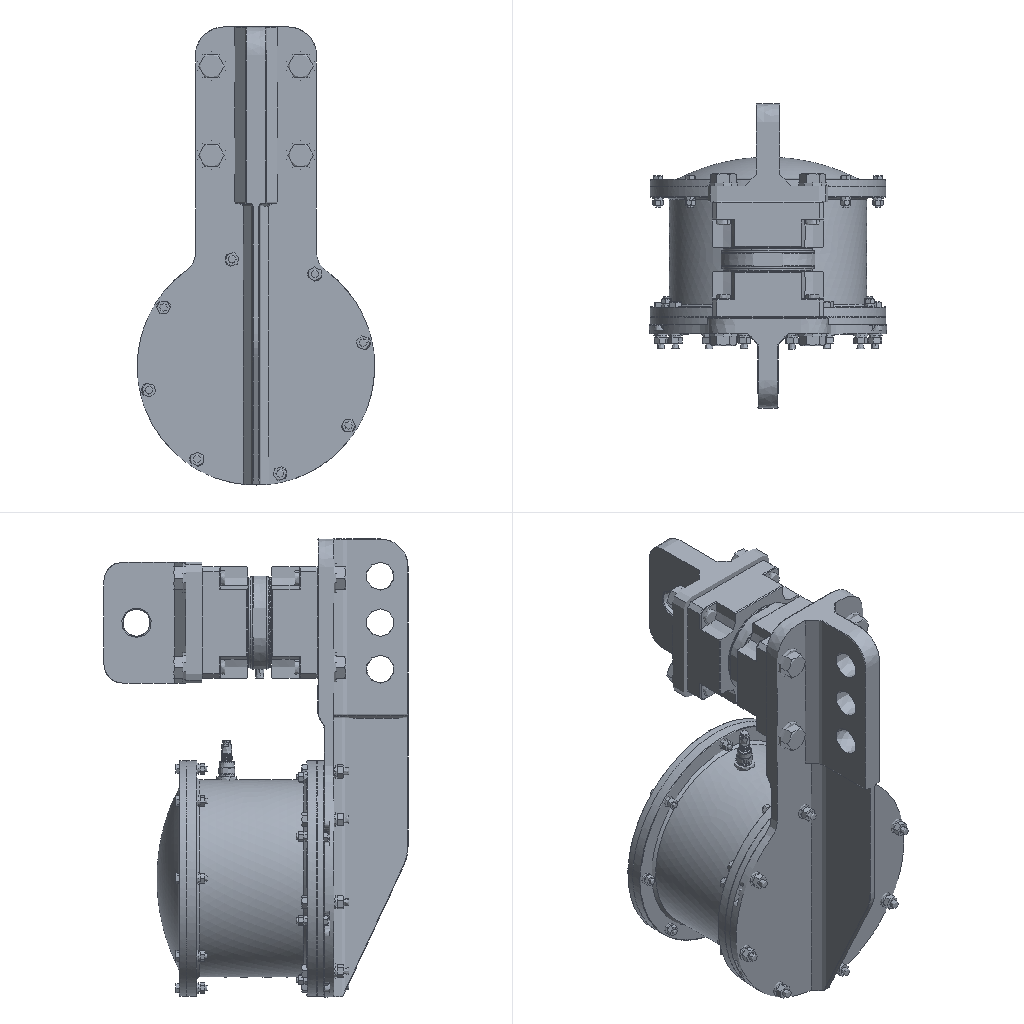Simulation study | ansys workbench
Set-up summary, first 219 of 917 lines:
category,name,step,type,value,unit,region
solver,ansys_mapdl
solver,version,,,22.2
units,MPA,,stated
analysis,deck,,static,static
load_step,requested,,,1
analysis,nlgeom,,,False
mesh,nodes,,,682109
mesh,elements,,,699995
element_type,ANSYS 187 (type 1),,solid,183
element_type,ANSYS 187 (type 2),,solid,17706
element_type,ANSYS 187 (type 3),,solid,59015
element_type,ANSYS 187 (type 4),,solid,6630
element_type,ANSYS 187 (type 5),,solid,23158
element_type,ANSYS 187 (type 6),,solid,2789
element_type,ANSYS 187 (type 7),,solid,7418
element_type,ANSYS 187 (type 8),,solid,4974
element_type,ANSYS 187 (type 9),,solid,5394
element_type,ANSYS 187 (type 10),,solid,2967
element_type,ANSYS 187 (type 11),,solid,1024
element_type,ANSYS 187 (type 12),,solid,918
element_type,ANSYS 187 (type 13),,solid,65195
element_type,ANSYS 187 (type 14),,solid,743
element_type,ANSYS 187 (type 15),,solid,719
element_type,ANSYS 187 (type 16),,solid,743
element_type,ANSYS 187 (type 17),,solid,716
element_type,ANSYS 187 (type 18),,solid,131786
element_type,ANSYS 187 (type 19),,solid,1036
element_type,ANSYS 187 (type 20),,solid,935
element_type,ANSYS 187 (type 21),,solid,48
element_type,ANSYS 187 (type 22),,solid,56
element_type,ANSYS 187 (type 23),,solid,234
element_type,ANSYS 187 (type 24),,solid,596
element_type,ANSYS 187 (type 25),,solid,599
element_type,ANSYS 187 (type 26),,solid,56
element_type,ANSYS 187 (type 27),,solid,48
element_type,ANSYS 187 (type 28),,solid,249
element_type,ANSYS 187 (type 29),,solid,561
element_type,ANSYS 187 (type 30),,solid,56
element_type,ANSYS 187 (type 31),,solid,48
element_type,ANSYS 187 (type 32),,solid,257
element_type,ANSYS 187 (type 33),,solid,588
element_type,ANSYS 187 (type 34),,solid,56
element_type,ANSYS 187 (type 35),,solid,48
element_type,ANSYS 187 (type 36),,solid,260
element_type,ANSYS 187 (type 37),,solid,577
element_type,ANSYS 187 (type 38),,solid,56
element_type,ANSYS 187 (type 39),,solid,48
element_type,ANSYS 187 (type 40),,solid,228
element_type,ANSYS 187 (type 41),,solid,659
element_type,ANSYS 187 (type 42),,solid,56
element_type,ANSYS 187 (type 43),,solid,48
element_type,ANSYS 187 (type 44),,solid,222
element_type,ANSYS 187 (type 45),,solid,586
element_type,ANSYS 187 (type 46),,solid,56
element_type,ANSYS 187 (type 47),,solid,48
element_type,ANSYS 187 (type 48),,solid,258
element_type,ANSYS 187 (type 49),,solid,593
element_type,ANSYS 187 (type 50),,solid,56
element_type,ANSYS 187 (type 51),,solid,48
element_type,ANSYS 187 (type 52),,solid,245
element_type,ANSYS 187 (type 53),,solid,215
element_type,ANSYS 187 (type 54),,solid,586
element_type,ANSYS 187 (type 55),,solid,58
element_type,ANSYS 187 (type 56),,solid,42
element_type,ANSYS 187 (type 57),,solid,47283
element_type,ANSYS 187 (type 58),,solid,647
element_type,ANSYS 187 (type 59),,solid,54
element_type,ANSYS 187 (type 60),,solid,54
element_type,ANSYS 187 (type 61),,solid,660
element_type,ANSYS 187 (type 62),,solid,54
element_type,ANSYS 187 (type 63),,solid,653
element_type,ANSYS 187 (type 64),,solid,54
element_type,ANSYS 187 (type 65),,solid,669
element_type,ANSYS 187 (type 66),,solid,670
element_type,ANSYS 187 (type 67),,solid,690
element_type,ANSYS 187 (type 68),,solid,661
element_type,ANSYS 187 (type 69),,solid,682
element_type,ANSYS 187 (type 70),,solid,48
element_type,ANSYS 187 (type 71),,solid,48
element_type,ANSYS 187 (type 72),,solid,48
element_type,ANSYS 187 (type 73),,solid,48
element_type,ANSYS 187 (type 74),,solid,554
element_type,ANSYS 187 (type 75),,solid,51
element_type,ANSYS 187 (type 76),,solid,48
element_type,ANSYS 187 (type 77),,solid,251
element_type,ANSYS 187 (type 78),,solid,48
element_type,ANSYS 187 (type 79),,solid,227
element_type,ANSYS 187 (type 80),,solid,51
element_type,ANSYS 187 (type 81),,solid,601
element_type,ANSYS 187 (type 82),,solid,48
element_type,ANSYS 187 (type 83),,solid,269
element_type,ANSYS 187 (type 84),,solid,51
element_type,ANSYS 187 (type 85),,solid,602
element_type,ANSYS 187 (type 86),,solid,48
element_type,ANSYS 187 (type 87),,solid,246
element_type,ANSYS 187 (type 88),,solid,51
element_type,ANSYS 187 (type 89),,solid,677
element_type,ANSYS 187 (type 90),,solid,48
element_type,ANSYS 187 (type 91),,solid,236
element_type,ANSYS 187 (type 92),,solid,51
element_type,ANSYS 187 (type 93),,solid,543
element_type,ANSYS 187 (type 94),,solid,48
element_type,ANSYS 187 (type 95),,solid,251
element_type,ANSYS 187 (type 96),,solid,51
element_type,ANSYS 187 (type 97),,solid,632
element_type,ANSYS 187 (type 98),,solid,48
element_type,ANSYS 187 (type 99),,solid,204
element_type,ANSYS 187 (type 100),,solid,51
element_type,ANSYS 187 (type 101),,solid,593
element_type,ANSYS 187 (type 102),,solid,48
element_type,ANSYS 187 (type 103),,solid,250
element_type,ANSYS 187 (type 104),,solid,51
element_type,ANSYS 187 (type 105),,solid,644
element_type,ANSYS 187 (type 106),,solid,233
element_type,ANSYS 187 (type 107),,solid,561
element_type,ANSYS 187 (type 108),,solid,42
element_type,ANSYS 187 (type 109),,solid,56
element_type,ANSYS 187 (type 110),,solid,261
element_type,ANSYS 187 (type 111),,solid,546
element_type,ANSYS 187 (type 112),,solid,42
element_type,ANSYS 187 (type 113),,solid,58
element_type,ANSYS 187 (type 114),,solid,217
element_type,ANSYS 187 (type 115),,solid,595
element_type,ANSYS 187 (type 116),,solid,42
element_type,ANSYS 187 (type 117),,solid,56
element_type,ANSYS 187 (type 118),,solid,218
element_type,ANSYS 187 (type 119),,solid,571
element_type,ANSYS 187 (type 120),,solid,42
element_type,ANSYS 187 (type 121),,solid,63
element_type,ANSYS 187 (type 122),,solid,222
element_type,ANSYS 187 (type 123),,solid,549
element_type,ANSYS 187 (type 124),,solid,42
element_type,ANSYS 187 (type 125),,solid,57
element_type,ANSYS 187 (type 126),,solid,236
element_type,ANSYS 187 (type 127),,solid,580
element_type,ANSYS 187 (type 128),,solid,42
element_type,ANSYS 187 (type 129),,solid,58
element_type,ANSYS 187 (type 130),,solid,259
element_type,ANSYS 187 (type 131),,solid,582
element_type,ANSYS 187 (type 132),,solid,42
element_type,ANSYS 187 (type 133),,solid,68
element_type,ANSYS 174 (type 134),,contact,357
element_type,ANSYS 170 (type 135),,target,357
element_type,ANSYS 174 (type 136),,contact,244
element_type,ANSYS 170 (type 137),,target,244
element_type,ANSYS 174 (type 138),,contact,225
element_type,ANSYS 170 (type 139),,target,225
element_type,ANSYS 174 (type 140),,contact,2467
element_type,ANSYS 170 (type 141),,target,2467
element_type,ANSYS 174 (type 142),,contact,60
element_type,ANSYS 170 (type 143),,target,60
element_type,ANSYS 174 (type 144),,contact,43
element_type,ANSYS 170 (type 145),,target,43
element_type,ANSYS 174 (type 146),,contact,37
element_type,ANSYS 170 (type 147),,target,37
element_type,ANSYS 174 (type 148),,contact,826
element_type,ANSYS 170 (type 149),,target,826
element_type,ANSYS 174 (type 150),,contact,84
element_type,ANSYS 170 (type 151),,target,84
element_type,ANSYS 174 (type 152),,contact,51
element_type,ANSYS 170 (type 153),,target,51
element_type,ANSYS 174 (type 154),,contact,58
element_type,ANSYS 170 (type 155),,target,58
element_type,ANSYS 174 (type 156),,contact,82
element_type,ANSYS 170 (type 157),,target,82
element_type,ANSYS 174 (type 158),,contact,58
element_type,ANSYS 170 (type 159),,target,58
element_type,ANSYS 174 (type 160),,contact,82
element_type,ANSYS 170 (type 161),,target,82
element_type,ANSYS 174 (type 162),,contact,51
element_type,ANSYS 170 (type 163),,target,51
element_type,ANSYS 174 (type 164),,contact,82
element_type,ANSYS 170 (type 165),,target,82
element_type,ANSYS 174 (type 166),,contact,16
element_type,ANSYS 170 (type 167),,target,16
element_type,ANSYS 174 (type 168),,contact,21
element_type,ANSYS 170 (type 169),,target,21
element_type,ANSYS 174 (type 170),,contact,22
element_type,ANSYS 170 (type 171),,target,22
element_type,ANSYS 174 (type 172),,contact,21
element_type,ANSYS 170 (type 173),,target,21
element_type,ANSYS 174 (type 174),,contact,21
element_type,ANSYS 170 (type 175),,target,21
element_type,ANSYS 174 (type 176),,contact,21
element_type,ANSYS 170 (type 177),,target,21
element_type,ANSYS 174 (type 178),,contact,21
element_type,ANSYS 170 (type 179),,target,21
element_type,ANSYS 174 (type 180),,contact,16
element_type,ANSYS 170 (type 181),,target,16
element_type,ANSYS 174 (type 182),,contact,58
element_type,ANSYS 170 (type 183),,target,58
element_type,ANSYS 174 (type 184),,contact,38
element_type,ANSYS 170 (type 185),,target,38
element_type,ANSYS 174 (type 186),,contact,52
element_type,ANSYS 170 (type 187),,target,52
element_type,ANSYS 174 (type 188),,contact,58
element_type,ANSYS 170 (type 189),,target,58
element_type,ANSYS 174 (type 190),,contact,33
element_type,ANSYS 170 (type 191),,target,33
element_type,ANSYS 174 (type 192),,contact,51
element_type,ANSYS 170 (type 193),,target,51
element_type,ANSYS 174 (type 194),,contact,58
element_type,ANSYS 170 (type 195),,target,58
element_type,ANSYS 174 (type 196),,contact,40
element_type,ANSYS 170 (type 197),,target,40
element_type,ANSYS 174 (type 198),,contact,48
element_type,ANSYS 170 (type 199),,target,48
element_type,ANSYS 174 (type 200),,contact,60
element_type,ANSYS 170 (type 201),,target,60
element_type,ANSYS 174 (type 202),,contact,42
element_type,ANSYS 170 (type 203),,target,42
element_type,ANSYS 174 (type 204),,contact,50
element_type,ANSYS 170 (type 205),,target,50
element_type,ANSYS 174 (type 206),,contact,56
element_type,ANSYS 170 (type 207),,target,56
element_type,ANSYS 174 (type 208),,contact,36
element_type,ANSYS 170 (type 209),,target,36
element_type,ANSYS 174 (type 210),,contact,52
Ansys APDL input file, long lists of numbers shortened:
/batch
/config,noeldb,1     ! force off writing results to database
*get,_wallstrt,active,,time,wall
! ANSYS input file written by Workbench version 2022 R2
! File used for geometry attach: D:\虚拟C盘\20260814\拖曳系统-湿端壳体-20260814.stp
/title,__--____ (A5)
! ****** Begin Custom Load Command Snippet ******
/COM, ACT Extensions:
/COM,     LSDYNA, 2022.2
/COM,/COM,     ANSYSMotion, 2022.2
/COM,
! ****** End   Custom Load Command Snippet ******
*DIM,_wb_ProjectScratch_dir,string,248
_wb_ProjectScratch_dir(1) = 'D:\虚拟C盘\20260815\_ProjectScratch\Scr2BC2\'
*DIM,_wb_SolverFiles_dir,string,248
_wb_SolverFiles_dir(1) = 'D:\虚拟C盘\20260815\仿真_files\dp0\SYS\MECH\'
*DIM,_wb_userfiles_dir,string,248
_wb_userfiles_dir(1) = 'D:\虚拟C盘\20260815\仿真_files\user_files\'
/com,--- Data in consistent NMM units. See Solving Units in the help system for more information.
/units,MPA
/nopr
/wb,file,start              !  signify a WB generated input file
/prep7
! Turn off shape checking because checks already performed inside WB mesher.
! See help system for more information.
SHPP,OFF,,NOWARN
/nolist
etcon,set             ! allow ANSYS to choose best KEYOP's for 180x elements, resets any applicable keyopt to MAPDL defaults
/com,*********** Nodes for the whole assembly ***********
nblock,3,,750319
(1i9,3e20.9e3)
   559923    -4.618127326E+00    -4.460000000E+01    -1.201185506E+04
! (682108 more lines like these left out)
-1
/wb,elem,start            !  set before creation of elements
/com,*********** Elements for Body 1 "____-____-20260814-FreeParts|song3688F4A9qif6" ***********
et,1,187
eblock,19,solid,,183
(19i9)
        1        1        1        1        0        0        0        0       10        0        1        4      107        5      106      137      144      133      136
! (365 more lines like these left out)
-1
/com,*********** Elements for Body 2 "____-____-20260814-FreeParts|song3688F4A9qif6[2]" ***********
et,2,187
eblock,19,solid,,17706
(19i9)
        2        2        2        2        0        0        0        0       10        0      184     3311     3564     5242     5167    23301    25029    23304    23303
! (35411 more lines like these left out)
-1
/com,*********** Elements for Body 3 "____-____-20260814-FreeParts|song3688F4A9qif6[3]" ***********
et,3,187
eblock,19,solid,,59015
(19i9)
        3        3        3        3        0        0        0        0       10        0    17890    36032    43716    38324    36340    81645    92824    81641    81639
! (118029 more lines like these left out)
-1
/com,*********** Elements for Body 4 "____-____-20260814-FreeParts|song3688F4A9qif6[4]" ***********
et,4,187
eblock,19,solid,,6630
(19i9)
        4        4        4        4        0        0        0        0       10        0    76905   128197   128208   128204   129438   132011   132093   132010   132019
! (13259 more lines like these left out)
-1
/com,*********** Elements for Body 5 "____-____-20260814-FreeParts|song3688F4A9qif6[5]" ***********
et,5,187
eblock,19,solid,,23158
(19i9)
        5        5        5        5        0        0        0        0       10        0    83535   143649   145248   144345   145242   169953   175001   169944   169952
! (46315 more lines like these left out)
-1
! (128 more sections like these left out)
/wb,elem,end               !  done creating elements
/com,*********** Send User Defined Coordinate System(s) ***********
csys,0
toffst,273.15,  ! Temperature offset from absolute zero
/com,*********** Set Reference Temperature ***********
tref,22.
/wb,mat,start              !  starting to send materials
/com,*********** Send Materials ***********
Temperature = 'TEMP' ! Temperature
MP,DENS,1,7.75e-09,	! tonne mm^-3
MP,ALPX,1,1.7e-05,	! C^-1
MP,C,1,480000000,	! mm^2 s^-2 C^-1
MP,KXX,1,15.1,	! tonne mm s^-3 C^-1
MP,RSVX,1,0.00077,	! ohm mm
MP,EX,1,193000,	! tonne s^-2 mm^-1
MP,NUXY,1,0.31,
MP,MURX,1,1,
Temperature = 'TEMP' ! Temperature
MP,DENS,2,7.75e-09,	! tonne mm^-3
MP,ALPX,2,1.7e-05,	! C^-1
MP,C,2,480000000,	! mm^2 s^-2 C^-1
MP,KXX,2,15.1,	! tonne mm s^-3 C^-1
MP,RSVX,2,0.00077,	! ohm mm
MP,EX,2,193000,	! tonne s^-2 mm^-1
MP,NUXY,2,0.31,
MP,MURX,2,1,
Temperature = 'TEMP' ! Temperature
MP,DENS,3,7.75e-09,	! tonne mm^-3
MP,ALPX,3,1.7e-05,	! C^-1
MP,C,3,480000000,	! mm^2 s^-2 C^-1
MP,KXX,3,15.1,	! tonne mm s^-3 C^-1
MP,RSVX,3,0.00077,	! ohm mm
MP,EX,3,193000,	! tonne s^-2 mm^-1
MP,NUXY,3,0.31,
MP,MURX,3,1,
Temperature = 'TEMP' ! Temperature
MP,DENS,4,7.75e-09,	! tonne mm^-3
MP,ALPX,4,1.7e-05,	! C^-1
MP,C,4,480000000,	! mm^2 s^-2 C^-1
MP,KXX,4,15.1,	! tonne mm s^-3 C^-1
MP,RSVX,4,0.00077,	! ohm mm
MP,EX,4,193000,	! tonne s^-2 mm^-1
MP,NUXY,4,0.31,
MP,MURX,4,1,
Temperature = 'TEMP' ! Temperature
MP,DENS,5,7.75e-09,	! tonne mm^-3
MP,ALPX,5,1.7e-05,	! C^-1
MP,C,5,480000000,	! mm^2 s^-2 C^-1
MP,KXX,5,15.1,	! tonne mm s^-3 C^-1
MP,RSVX,5,0.00077,	! ohm mm
MP,EX,5,193000,	! tonne s^-2 mm^-1
MP,NUXY,5,0.31,
MP,MURX,5,1,
Temperature = 'TEMP' ! Temperature
MP,DENS,6,7.75e-09,	! tonne mm^-3
MP,ALPX,6,1.7e-05,	! C^-1
MP,C,6,480000000,	! mm^2 s^-2 C^-1
MP,KXX,6,15.1,	! tonne mm s^-3 C^-1
MP,RSVX,6,0.00077,	! ohm mm
MP,EX,6,193000,	! tonne s^-2 mm^-1
MP,NUXY,6,0.31,
MP,MURX,6,1,
Temperature = 'TEMP' ! Temperature
MP,DENS,7,7.75e-09,	! tonne mm^-3
MP,ALPX,7,1.7e-05,	! C^-1
MP,C,7,480000000,	! mm^2 s^-2 C^-1
MP,KXX,7,15.1,	! tonne mm s^-3 C^-1
MP,RSVX,7,0.00077,	! ohm mm
MP,EX,7,193000,	! tonne s^-2 mm^-1
MP,NUXY,7,0.31,
MP,MURX,7,1,
Temperature = 'TEMP' ! Temperature
MP,DENS,8,7.75e-09,	! tonne mm^-3
MP,ALPX,8,1.7e-05,	! C^-1
MP,C,8,480000000,	! mm^2 s^-2 C^-1
MP,KXX,8,15.1,	! tonne mm s^-3 C^-1
MP,RSVX,8,0.00077,	! ohm mm
MP,EX,8,193000,	! tonne s^-2 mm^-1
MP,NUXY,8,0.31,
MP,MURX,8,1,
Temperature = 'TEMP' ! Temperature
MP,DENS,9,7.75e-09,	! tonne mm^-3
MP,ALPX,9,1.7e-05,	! C^-1
MP,C,9,480000000,	! mm^2 s^-2 C^-1
MP,KXX,9,15.1,	! tonne mm s^-3 C^-1
MP,RSVX,9,0.00077,	! ohm mm
MP,EX,9,193000,	! tonne s^-2 mm^-1
! (1118 more lines like these left out)
/wb,mat,end                !  done sending materials
!************************* Model Summary ********************
!____-____-20260814-FreeParts|song3688F4A9qif6,	不锈钢,	matid,	1
!____-____-20260814-FreeParts|song3688F4A9qif6[2],	不锈钢,	matid,	2
!____-____-20260814-FreeParts|song3688F4A9qif6[3],	不锈钢,	matid,	3
! (132 more lines like these left out)
*get,_xmin,node,,mnloc,x
*get,_ymin,node,,mnloc,y
*get,_zmin,node,,mnloc,z
*get,_xmax,node,,mxloc,x
*get,_ymax,node,,mxloc,y
*get,_zmax,node,,mxloc,z
_ASMDIAG=(_xmax-_xmin)*(_xmax-_xmin)+(_ymax-_ymin)*(_ymax-_ymin)+(_zmax-_zmin)*(_zmax-_zmin)
_ASMDIAG=SQRT(_ASMDIAG)
/wb,contact,start          !  starting to send contact
/com,*********** Create Contact "接触区域" ***********
/com,            Real Constant Set For Above Contact Is 135 & 134
*set,tid,135
*set,cid,134
r,tid
r,cid
et,tid,170
et,cid,174
eblock,10,,,210
(15i9)
   534566      135      135      135        0       32       33       34       34      304      310       34      305
! (209 more lines like these left out)
-1
eblock,10,,,210
(15i9)
   534776      134      134      134        0       32       33       34       34      304      310       34      305
! (209 more lines like these left out)
-1
eblock,10,,,147
(15i9)
   534986      134      135      134        0   127959   127962   127992   127992   130079   130101   127992   130080
! (146 more lines like these left out)
-1
eblock,10,,,147
(15i9)
   535133      135      134      135        0   127959   127962   127992   127992   130079   130101   127992   130080
! (146 more lines like these left out)
-1
keyo,cid,8,2               ! auto create asymmetric contact (from Program Controlled setting)
keyo,cid,10,0              ! adjust contact stiffness each NR iteration (from Program Controlled setting)
keyo,cid,12,5              ! bonded always
keyo,cid,18,1              ! small sliding turned on by application
keyo,cid,2,0               ! augmented Lagrange (from Program Controlled setting)
keyo,cid,4,0               ! on Gauss point (from Program Controlled setting)
keyo,cid,9,1               ! ignore initial gaps/penetration
keyo,cid,7,0               ! No Prediction
rmod,tid,3,10.      ! FKN
rmod,tid,5,0.       ! ICONT
rmod,tid,6,0.       ! PINB
rmod,tid,10,0.      ! CNOF
rmod,tid,12,0.      ! FKT
rmod,tid,36,422     ! WB DSID
rmod,cid,3,10.      ! FKN
rmod,cid,5,0.       ! ICONT
rmod,cid,6,0.       ! PINB
rmod,cid,10,0.      ! CNOF
rmod,cid,12,0.      ! FKT
rmod,cid,36,422     ! WB DSID
/com,*********** Create Contact "接触区域 2" ***********
/com,            Real Constant Set For Above Contact Is 137 & 136
*set,tid,137
*set,cid,136
r,tid
r,cid
et,tid,170
et,cid,174
eblock,10,,,210
(15i9)
   535280      137      137      137        0       32       33       34       34      304      310       34      305
! (209 more lines like these left out)
-1
eblock,10,,,210
(15i9)
   535490      136      136      136        0       32       33       34       34      304      310       34      305
! (209 more lines like these left out)
-1
eblock,10,,,34
(15i9)
   535700      136      137      136        0   194769   194795   194773   194773   198184   198218   194773   198180
! (33 more lines like these left out)
-1
eblock,10,,,34
(15i9)
   535734      137      136      137        0   194769   194795   194773   194773   198184   198218   194773   198180
! (33 more lines like these left out)
-1
keyo,cid,8,2               ! auto create asymmetric contact (from Program Controlled setting)
keyo,cid,10,0              ! adjust contact stiffness each NR iteration (from Program Controlled setting)
keyo,cid,12,5              ! bonded always
keyo,cid,18,1              ! small sliding turned on by application
keyo,cid,2,0               ! augmented Lagrange (from Program Controlled setting)
keyo,cid,4,0               ! on Gauss point (from Program Controlled setting)
keyo,cid,9,1               ! ignore initial gaps/penetration
keyo,cid,7,0               ! No Prediction
rmod,tid,3,10.      ! FKN
rmod,tid,5,0.       ! ICONT
rmod,tid,6,0.       ! PINB
rmod,tid,10,0.      ! CNOF
rmod,tid,12,0.      ! FKT
rmod,tid,36,425     ! WB DSID
rmod,cid,3,10.      ! FKN
rmod,cid,5,0.       ! ICONT
rmod,cid,6,0.       ! PINB
rmod,cid,10,0.      ! CNOF
rmod,cid,12,0.      ! FKT
rmod,cid,36,425     ! WB DSID
/com,*********** Create Contact "接触区域 3" ***********
/com,            Real Constant Set For Above Contact Is 139 & 138
*set,tid,139
*set,cid,138
r,tid
r,cid
et,tid,170
et,cid,174
eblock,10,,,210
(15i9)
   535768      139      139      139        0       32       33       34       34      304      310       34      305
! (209 more lines like these left out)
-1
eblock,10,,,210
(15i9)
   535978      138      138      138        0       32       33       34       34      304      310       34      305
! (209 more lines like these left out)
-1
eblock,10,,,15
(15i9)
   536188      138      139      138        0   337473   337482   337478   337478   372149   372163   337478   372148
! (14 more lines like these left out)
-1
eblock,10,,,15
(15i9)
   536203      139      138      139        0   337473   337482   337478   337478   372149   372163   337478   372148
! (14 more lines like these left out)
-1
keyo,cid,8,2               ! auto create asymmetric contact (from Program Controlled setting)
keyo,cid,10,0              ! adjust contact stiffness each NR iteration (from Program Controlled setting)
keyo,cid,12,5              ! bonded always
keyo,cid,18,1              ! small sliding turned on by application
keyo,cid,2,0               ! augmented Lagrange (from Program Controlled setting)
keyo,cid,4,0               ! on Gauss point (from Program Controlled setting)
keyo,cid,9,1               ! ignore initial gaps/penetration
keyo,cid,7,0               ! No Prediction
rmod,tid,3,10.      ! FKN
rmod,tid,5,0.       ! ICONT
rmod,tid,6,0.       ! PINB
rmod,tid,10,0.      ! CNOF
rmod,tid,12,0.      ! FKT
rmod,tid,36,428     ! WB DSID
rmod,cid,3,10.      ! FKN
rmod,cid,5,0.       ! ICONT
rmod,cid,6,0.       ! PINB
rmod,cid,10,0.      ! CNOF
rmod,cid,12,0.      ! FKT
rmod,cid,36,428     ! WB DSID
/com,*********** Create Contact "接触区域 4" ***********
/com,            Real Constant Set For Above Contact Is 141 & 140
*set,tid,141
*set,cid,140
r,tid
r,cid
et,tid,170
et,cid,174
eblock,10,,,1245
(15i9)
   536218      141      141      141        0     2131     2441     2225     2225    17071    17903     2225    17068
! (1244 more lines like these left out)
-1
eblock,10,,,1245
(15i9)
   537463      140      140      140        0     2131     2441     2225     2225    17071    17903     2225    17068
! (1244 more lines like these left out)
-1
eblock,10,,,1222
(15i9)
   538708      140      141      140        0   230052   230176   230315   230315   292041   293052   230315   292043
! (1221 more lines like these left out)
-1
eblock,10,,,1222
(15i9)
   539930      141      140      141        0   230052   230176   230315   230315   292041   293052   230315   292043
! (1221 more lines like these left out)
-1
keyo,cid,8,2               ! auto create asymmetric contact (from Program Controlled setting)
keyo,cid,10,0              ! adjust contact stiffness each NR iteration (from Program Controlled setting)
keyo,cid,12,5              ! bonded always
keyo,cid,18,1              ! small sliding turned on by application
keyo,cid,2,0               ! augmented Lagrange (from Program Controlled setting)
keyo,cid,4,0               ! on Gauss point (from Program Controlled setting)
keyo,cid,9,1               ! ignore initial gaps/penetration
keyo,cid,7,0               ! No Prediction
rmod,tid,3,10.      ! FKN
rmod,tid,5,0.       ! ICONT
rmod,tid,6,0.       ! PINB
rmod,tid,10,0.      ! CNOF
rmod,tid,12,0.      ! FKT
rmod,tid,36,431     ! WB DSID
rmod,cid,3,10.      ! FKN
rmod,cid,5,0.       ! ICONT
rmod,cid,6,0.       ! PINB
rmod,cid,10,0.      ! CNOF
rmod,cid,12,0.      ! FKT
rmod,cid,36,431     ! WB DSID
/com,*********** Create Contact "接触区域 5" ***********
/com,            Real Constant Set For Above Contact Is 143 & 142
*set,tid,143
*set,cid,142
r,tid
r,cid
et,tid,170
et,cid,174
eblock,10,,,24
(15i9)
   541152      143      143      143        0      654      651     3280     3280     6519     6521     3280     6540
! (23 more lines like these left out)
-1
eblock,10,,,24
(15i9)
   541176      142      142      142        0      654      651     3280     3280     6519     6521     3280     6540
! (23 more lines like these left out)
-1
eblock,10,,,36
(15i9)
   541200      142      143      142        0   566834   566898   566894   566894   567248   567559   566894   567247
! (35 more lines like these left out)
-1
eblock,10,,,36
(15i9)
   541236      143      142      143        0   566834   566898   566894   566894   567248   567559   566894   567247
! (35 more lines like these left out)
-1
keyo,cid,8,2               ! auto create asymmetric contact (from Program Controlled setting)
keyo,cid,10,0              ! adjust contact stiffness each NR iteration (from Program Controlled setting)
keyo,cid,12,5              ! bonded always
keyo,cid,18,1              ! small sliding turned on by application
keyo,cid,2,0               ! augmented Lagrange (from Program Controlled setting)
keyo,cid,4,0               ! on Gauss point (from Program Controlled setting)
keyo,cid,9,1               ! ignore initial gaps/penetration
keyo,cid,7,0               ! No Prediction
rmod,tid,3,10.      ! FKN
rmod,tid,5,0.       ! ICONT
rmod,tid,6,0.       ! PINB
rmod,tid,10,0.      ! CNOF
rmod,tid,12,0.      ! FKT
rmod,tid,36,434     ! WB DSID
rmod,cid,3,10.      ! FKN
rmod,cid,5,0.       ! ICONT
rmod,cid,6,0.       ! PINB
rmod,cid,10,0.      ! CNOF
rmod,cid,12,0.      ! FKT
rmod,cid,36,434     ! WB DSID
! (313 more sections like these left out)
/wb,contact,end            !  done creating contacts
/golist
/wb,load,start             !  starting to send loads
/com,*********** Fixed Supports ***********
CMBLOCK,_FIXEDSU,NODE,      526
(8i10)
      1497      1498      1499      1500      1501      1502      1503      1504
! (65 more lines like these left out)
cmsel,s,_FIXEDSU
d,all,all
nsel,all
/com,*********** Define Pressure Using Surface Effect Elements "__" ***********
et,770,154
eblock,10,,,125136
(15i9)
   697238      770      770      770        0       32       33       34       34      304      310       34      305
! (125135 more lines like these left out)
-1
esel,s,type,,770
keyop,770,7,0                ! Use deformed area for application of load
esel,all
/com,*********** Define Pressure Using Surface Effect Elements "__ 2" ***********
et,771,154
eblock,10,,,2758
(15i9)
   822374      771      771      771        0   350838   350839   350973   350973   467467   467478   350973   467469
! (2757 more lines like these left out)
-1
esel,s,type,,771
keyop,771,7,0                ! Use deformed area for application of load
esel,all
esel,all
/gst,on,on
fini
*get,_numnode,node,0,count
*get,_numelem,elem,0,count
*get, _MAXELEMNUM, elem, 0, NUM, MAX
*get, _MAXNODENUM, node, 0, NUM, MAX
*get, _MAXELEMTYPE, etyp, 0, NUM, MAX
*get, _MAXREALCONST, rcon, 0, NUM, MAX
/go
/wb,load,end               !  done creating loads
/com,--- Number of total nodes = %_numnode%
/com,--- Number of contact elements = 290566
/com,--- Number of spring elements = 0
/com,--- Number of bearing elements = 0
/com,--- Number of solid elements = 409429
/com,--- Number of condensed parts = 0
/com,--- Number of total elements = %_numelem%
*get,_wallbsol,active,,time,wall
/com,****************************************************************************
/com,*************************    SOLUTION       ********************************
/com,****************************************************************************
/solu
antype,0                   ! static analysis
_thickRatio=0.323   ! Ratio of thick parts in the model
eqsl,sparse,,,,,1
cntr,print,1               ! print out contact info and also make no initial contact an error
cntr,out,yes               ! write contact output to file.cmn due to many contact pairs present
dmpoption,emat,no             ! Don't combine emat file for DANSYS
dmpoption,esav,no             ! Don't combine esav file for DANSYS
nldiag,cont,iter           ! print out contact info each equilibrium iteration
rescontrol,,none                 ! Do not keep any restart files
/com,****************************************************
/com,******************* SOLVE FOR LS 1 OF 1 ****************
esel,s,type,,770
nsle
sf,all,pres,1.5
esel,s,type,,771
nsle
sf,all,pres,0.1013
nsel,all
esel,all
esel,all
/nopr
/gopr
nsub,1,1,1
time,1.
outres,erase
outres,all,none
outres,nsol,all,
outres,rsol,all
outres,eangl,all
outres,etmp,all
outres,veng,all
outres,strs,all,
outres,epel,all,
outres,eppl,all,
outres,cont,all,
! *********** WB SOLVE COMMAND ***********
! check interactive state
*get,ANSINTER_,active,,int
*if,ANSINTER_,ne,0,then
/eof
*endif
solve
/com *************** Write FE CONNECTORS *********
CEWRITE,file,ce,,INTE
/com,****************************************************
/com,*************** FINISHED SOLVE FOR LS 1 *************
*get,_wallasol,active,,time,wall
/nopr
*get,_numnode,node,0,count
*get,_numelem,elem,0,count
*get, _MAXELEMNUM, elem, 0, NUM, MAX
*get, _MAXNODENUM, node, 0, NUM, MAX,,,INTERNAL
*get, _MAXELEMTYPE, etyp, 0, NUM, MAX
*get, _MAXREALCONST, rcon, 0, NUM, MAX
*get,_NSOLTHREADS,active,0,ntfs
*get,_NSOLPROCESSES,active,0,npfs
/gopr
/post1
xmlo,ENCODING,ISO-8859-1
xmlo,parm
/xml,parm,xml
fini
/gopr
*get,_walldone,active,,time,wall
_preptime=(_wallbsol-_wallstrt)*3600
_solvtime=(_wallasol-_wallbsol)*3600
_posttime=(_walldone-_wallasol)*3600
_totaltim=(_walldone-_wallstrt)*3600
*get,_dlbratio,active,0,solu,dlbr
*get,_combtime,active,0,solu,comb
*get,_ssmode,active,0,solu,ssmm
*get,_ndofs,active,0,solu,ndof
*get,_sol_end_time,active,0,set,time
*if,_sol_end_time,eq,1.,then
/fclean				!clean distributed files
*endif
/com,--- Total number of nodes = %_numnode%
/com,--- Total number of elements = %_numelem%
/com,--- Element load balance ratio = %_dlbratio%
/com,--- Time to combine distributed files = %_combtime%
/com,--- Sparse memory mode = %_ssmode%
/com,--- Number of DOF = %_ndofs%
/wb,file,end               ! done with WB generated input
Results summary:
result,analysis,,,static
result,last_loadstep,,,1
result,primary field,,,displacement
result,reaction total,1,FX,-1.6e-05,N
result,reaction total,1,FY,1.2e-05,N
result,reaction total,1,FZ,8.264,N
result,mass,,,0.05295,"NMM: mm, ton, N, s, mV, mA, degC"